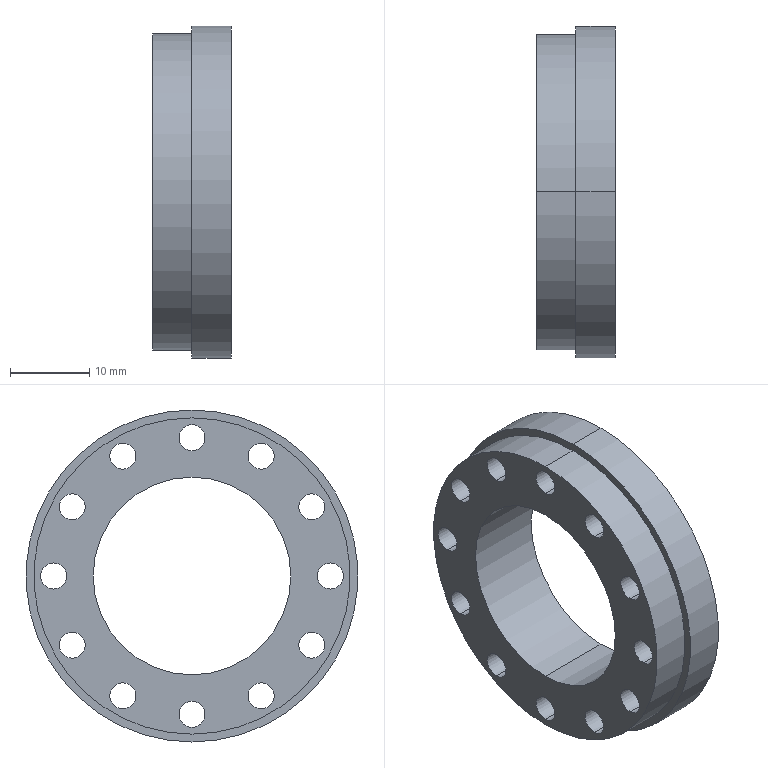Part | SolidWorks | features HoleWzd 1, Revolution 1 | 1 solid | 33 faces | box 9.95 x 42 x 42 mm | volume 7242 mm3 | cylinder 30 | plane 3 | commonest cylinder face diameters 3.3 x24 25 x2 40 x2 42 x2
STEP:
#1=CARTESIAN_POINT('',(0.,17.5,1.65));
#2=VERTEX_POINT('',#1);
#3=CARTESIAN_POINT('',(0.,17.5,-1.65));
#4=VERTEX_POINT('',#3);
#5=CARTESIAN_POINT('',(0.,17.5,0.));
#6=DIRECTION('',(1.,0.,0.));
#7=DIRECTION('',(0.,0.,-1.));
#8=AXIS2_PLACEMENT_3D('',#5,#6,#7);
#9=CIRCLE('',#8,1.65);
#10=EDGE_CURVE('',#2,#4,#9,.T.);
#11=ORIENTED_EDGE('',*,*,#10,.F.);
#12=CARTESIAN_POINT('',(9.95,17.5,1.65));
#13=VERTEX_POINT('',#12);
#14=CARTESIAN_POINT('',(9.95,17.5,1.65));
#15=DIRECTION('',(1.,0.,0.));
#16=VECTOR('',#15,1000.);
#17=LINE('',#14,#16);
#18=EDGE_CURVE('',#2,#13,#17,.T.);
#19=ORIENTED_EDGE('',*,*,#18,.T.);
#20=CARTESIAN_POINT('',(9.95,17.5,-1.65));
#21=VERTEX_POINT('',#20);
#22=CARTESIAN_POINT('',(9.95,17.5,0.));
#23=DIRECTION('',(1.,0.,0.));
#24=DIRECTION('',(0.,0.,-1.));
#25=AXIS2_PLACEMENT_3D('',#22,#23,#24);
#26=CIRCLE('',#25,1.65);
#27=EDGE_CURVE('',#13,#21,#26,.T.);
#28=ORIENTED_EDGE('',*,*,#27,.T.);
#29=CARTESIAN_POINT('',(9.95,17.5,-1.65));
#30=DIRECTION('',(1.,0.,0.));
#31=VECTOR('',#30,1000.);
#32=LINE('',#29,#31);
#33=EDGE_CURVE('',#4,#21,#32,.T.);
#34=ORIENTED_EDGE('',*,*,#33,.F.);
#35=EDGE_LOOP('',(#11,#19,#28,#34));
#36=FACE_OUTER_BOUND('',#35,.T.);
#37=CARTESIAN_POINT('',(9.95,17.5,0.));
#38=DIRECTION('',(1.,0.,0.));
#39=DIRECTION('',(0.,0.,-1.));
#40=AXIS2_PLACEMENT_3D('',#37,#38,#39);
#41=CYLINDRICAL_SURFACE('',#40,1.65);
#42=ADVANCED_FACE('',(#36),#41,.F.);
#43=CARTESIAN_POINT('',(0.,15.155,-7.1));
#44=VERTEX_POINT('',#43);
#45=CARTESIAN_POINT('',(0.,15.155,-10.4));
#46=VERTEX_POINT('',#45);
#47=CARTESIAN_POINT('',(0.,15.155,-8.75));
#48=DIRECTION('',(1.,0.,0.));
#49=DIRECTION('',(0.,0.,-1.));
#50=AXIS2_PLACEMENT_3D('',#47,#48,#49);
#51=CIRCLE('',#50,1.65);
#52=EDGE_CURVE('',#44,#46,#51,.T.);
#53=ORIENTED_EDGE('',*,*,#52,.F.);
#54=CARTESIAN_POINT('',(9.95,15.155,-7.1));
#55=VERTEX_POINT('',#54);
#56=CARTESIAN_POINT('',(9.95,15.155,-7.1));
#57=DIRECTION('',(1.,0.,0.));
#58=VECTOR('',#57,1000.);
#59=LINE('',#56,#58);
#60=EDGE_CURVE('',#44,#55,#59,.T.);
#61=ORIENTED_EDGE('',*,*,#60,.T.);
#62=CARTESIAN_POINT('',(9.95,15.155,-10.4));
#63=VERTEX_POINT('',#62);
#64=CARTESIAN_POINT('',(9.95,15.155,-8.75));
#65=DIRECTION('',(1.,0.,0.));
#66=DIRECTION('',(0.,0.,-1.));
#67=AXIS2_PLACEMENT_3D('',#64,#65,#66);
#68=CIRCLE('',#67,1.65);
#69=EDGE_CURVE('',#55,#63,#68,.T.);
#70=ORIENTED_EDGE('',*,*,#69,.T.);
#71=CARTESIAN_POINT('',(9.95,15.155,-10.4));
#72=DIRECTION('',(1.,0.,0.));
#73=VECTOR('',#72,1000.);
#74=LINE('',#71,#73);
#75=EDGE_CURVE('',#46,#63,#74,.T.);
#76=ORIENTED_EDGE('',*,*,#75,.F.);
#77=EDGE_LOOP('',(#53,#61,#70,#76));
#78=FACE_OUTER_BOUND('',#77,.T.);
#79=CARTESIAN_POINT('',(9.95,15.155,-8.75));
#80=DIRECTION('',(1.,0.,0.));
#81=DIRECTION('',(0.,0.,-1.));
#82=AXIS2_PLACEMENT_3D('',#79,#80,#81);
#83=CYLINDRICAL_SURFACE('',#82,1.65);
#84=ADVANCED_FACE('',(#78),#83,.F.);
#85=CARTESIAN_POINT('',(0.,8.75,-13.505));
#86=VERTEX_POINT('',#85);
#87=CARTESIAN_POINT('',(0.,8.75,-16.805));
#88=VERTEX_POINT('',#87);
#89=CARTESIAN_POINT('',(0.,8.75,-15.155));
#90=DIRECTION('',(1.,0.,0.));
#91=DIRECTION('',(0.,0.,-1.));
#92=AXIS2_PLACEMENT_3D('',#89,#90,#91);
#93=CIRCLE('',#92,1.65);
#94=EDGE_CURVE('',#86,#88,#93,.T.);
#95=ORIENTED_EDGE('',*,*,#94,.F.);
#96=CARTESIAN_POINT('',(9.95,8.75,-13.505));
#97=VERTEX_POINT('',#96);
#98=CARTESIAN_POINT('',(9.95,8.75,-13.505));
#99=DIRECTION('',(1.,0.,0.));
#100=VECTOR('',#99,1000.);
#101=LINE('',#98,#100);
#102=EDGE_CURVE('',#86,#97,#101,.T.);
#103=ORIENTED_EDGE('',*,*,#102,.T.);
#104=CARTESIAN_POINT('',(9.95,8.75,-16.805));
#105=VERTEX_POINT('',#104);
#106=CARTESIAN_POINT('',(9.95,8.75,-15.155));
#107=DIRECTION('',(1.,0.,0.));
#108=DIRECTION('',(0.,0.,-1.));
#109=AXIS2_PLACEMENT_3D('',#106,#107,#108);
#110=CIRCLE('',#109,1.65);
#111=EDGE_CURVE('',#97,#105,#110,.T.);
#112=ORIENTED_EDGE('',*,*,#111,.T.);
#113=CARTESIAN_POINT('',(9.95,8.75,-16.805));
#114=DIRECTION('',(1.,0.,0.));
#115=VECTOR('',#114,1000.);
#116=LINE('',#113,#115);
#117=EDGE_CURVE('',#88,#105,#116,.T.);
#118=ORIENTED_EDGE('',*,*,#117,.F.);
#119=EDGE_LOOP('',(#95,#103,#112,#118));
#120=FACE_OUTER_BOUND('',#119,.T.);
#121=CARTESIAN_POINT('',(9.95,8.75,-15.155));
#122=DIRECTION('',(1.,0.,0.));
#123=DIRECTION('',(0.,0.,-1.));
#124=AXIS2_PLACEMENT_3D('',#121,#122,#123);
#125=CYLINDRICAL_SURFACE('',#124,1.65);
#126=ADVANCED_FACE('',(#120),#125,.F.);
#127=CARTESIAN_POINT('',(0.,0.,-15.85));
#128=VERTEX_POINT('',#127);
#129=CARTESIAN_POINT('',(0.,0.,-19.15));
#130=VERTEX_POINT('',#129);
#131=CARTESIAN_POINT('',(0.,0.,-17.5));
#132=DIRECTION('',(1.,0.,0.));
#133=DIRECTION('',(0.,0.,-1.));
#134=AXIS2_PLACEMENT_3D('',#131,#132,#133);
#135=CIRCLE('',#134,1.65);
#136=EDGE_CURVE('',#128,#130,#135,.T.);
#137=ORIENTED_EDGE('',*,*,#136,.F.);
#138=CARTESIAN_POINT('',(9.95,0.,-15.85));
#139=VERTEX_POINT('',#138);
#140=CARTESIAN_POINT('',(9.95,0.,-15.85));
#141=DIRECTION('',(1.,0.,0.));
#142=VECTOR('',#141,1000.);
#143=LINE('',#140,#142);
#144=EDGE_CURVE('',#128,#139,#143,.T.);
#145=ORIENTED_EDGE('',*,*,#144,.T.);
#146=CARTESIAN_POINT('',(9.95,0.,-19.15));
#147=VERTEX_POINT('',#146);
#148=CARTESIAN_POINT('',(9.95,0.,-17.5));
#149=DIRECTION('',(1.,0.,0.));
#150=DIRECTION('',(0.,0.,-1.));
#151=AXIS2_PLACEMENT_3D('',#148,#149,#150);
#152=CIRCLE('',#151,1.65);
#153=EDGE_CURVE('',#139,#147,#152,.T.);
#154=ORIENTED_EDGE('',*,*,#153,.T.);
#155=CARTESIAN_POINT('',(9.95,0.,-19.15));
#156=DIRECTION('',(1.,0.,0.));
#157=VECTOR('',#156,1000.);
#158=LINE('',#155,#157);
#159=EDGE_CURVE('',#130,#147,#158,.T.);
#160=ORIENTED_EDGE('',*,*,#159,.F.);
#161=EDGE_LOOP('',(#137,#145,#154,#160));
#162=FACE_OUTER_BOUND('',#161,.T.);
#163=CARTESIAN_POINT('',(9.95,0.,-17.5));
#164=DIRECTION('',(1.,0.,0.));
#165=DIRECTION('',(0.,0.,-1.));
#166=AXIS2_PLACEMENT_3D('',#163,#164,#165);
#167=CYLINDRICAL_SURFACE('',#166,1.65);
#168=ADVANCED_FACE('',(#162),#167,.F.);
#169=CARTESIAN_POINT('',(0.,-8.75,-13.505));
#170=VERTEX_POINT('',#169);
#171=CARTESIAN_POINT('',(0.,-8.75,-16.805));
#172=VERTEX_POINT('',#171);
#173=CARTESIAN_POINT('',(0.,-8.75,-15.155));
#174=DIRECTION('',(1.,0.,0.));
#175=DIRECTION('',(0.,0.,-1.));
#176=AXIS2_PLACEMENT_3D('',#173,#174,#175);
#177=CIRCLE('',#176,1.65);
#178=EDGE_CURVE('',#170,#172,#177,.T.);
#179=ORIENTED_EDGE('',*,*,#178,.F.);
#180=CARTESIAN_POINT('',(9.95,-8.75,-13.505));
#181=VERTEX_POINT('',#180);
#182=CARTESIAN_POINT('',(9.95,-8.75,-13.505));
#183=DIRECTION('',(1.,0.,0.));
#184=VECTOR('',#183,1000.);
#185=LINE('',#182,#184);
#186=EDGE_CURVE('',#170,#181,#185,.T.);
#187=ORIENTED_EDGE('',*,*,#186,.T.);
#188=CARTESIAN_POINT('',(9.95,-8.75,-16.805));
#189=VERTEX_POINT('',#188);
#190=CARTESIAN_POINT('',(9.95,-8.75,-15.155));
#191=DIRECTION('',(1.,0.,0.));
#192=DIRECTION('',(0.,0.,-1.));
#193=AXIS2_PLACEMENT_3D('',#190,#191,#192);
#194=CIRCLE('',#193,1.65);
#195=EDGE_CURVE('',#181,#189,#194,.T.);
#196=ORIENTED_EDGE('',*,*,#195,.T.);
#197=CARTESIAN_POINT('',(9.95,-8.75,-16.805));
#198=DIRECTION('',(1.,0.,0.));
#199=VECTOR('',#198,1000.);
#200=LINE('',#197,#199);
#201=EDGE_CURVE('',#172,#189,#200,.T.);
#202=ORIENTED_EDGE('',*,*,#201,.F.);
#203=EDGE_LOOP('',(#179,#187,#196,#202));
#204=FACE_OUTER_BOUND('',#203,.T.);
#205=CARTESIAN_POINT('',(9.95,-8.75,-15.155));
#206=DIRECTION('',(1.,0.,0.));
#207=DIRECTION('',(0.,0.,-1.));
#208=AXIS2_PLACEMENT_3D('',#205,#206,#207);
#209=CYLINDRICAL_SURFACE('',#208,1.65);
#210=ADVANCED_FACE('',(#204),#209,.F.);
#211=CARTESIAN_POINT('',(0.,-15.155,-7.1));
#212=VERTEX_POINT('',#211);
#213=CARTESIAN_POINT('',(0.,-15.155,-10.4));
#214=VERTEX_POINT('',#213);
#215=CARTESIAN_POINT('',(0.,-15.155,-8.75));
#216=DIRECTION('',(1.,0.,0.));
#217=DIRECTION('',(0.,0.,-1.));
#218=AXIS2_PLACEMENT_3D('',#215,#216,#217);
#219=CIRCLE('',#218,1.65);
#220=EDGE_CURVE('',#212,#214,#219,.T.);
#221=ORIENTED_EDGE('',*,*,#220,.F.);
#222=CARTESIAN_POINT('',(9.95,-15.155,-7.1));
#223=VERTEX_POINT('',#222);
#224=CARTESIAN_POINT('',(9.95,-15.155,-7.1));
#225=DIRECTION('',(1.,0.,0.));
#226=VECTOR('',#225,1000.);
#227=LINE('',#224,#226);
#228=EDGE_CURVE('',#212,#223,#227,.T.);
#229=ORIENTED_EDGE('',*,*,#228,.T.);
#230=CARTESIAN_POINT('',(9.95,-15.155,-10.4));
#231=VERTEX_POINT('',#230);
#232=CARTESIAN_POINT('',(9.95,-15.155,-8.75));
#233=DIRECTION('',(1.,0.,0.));
#234=DIRECTION('',(0.,0.,-1.));
#235=AXIS2_PLACEMENT_3D('',#232,#233,#234);
#236=CIRCLE('',#235,1.65);
#237=EDGE_CURVE('',#223,#231,#236,.T.);
#238=ORIENTED_EDGE('',*,*,#237,.T.);
#239=CARTESIAN_POINT('',(9.95,-15.155,-10.4));
#240=DIRECTION('',(1.,0.,0.));
#241=VECTOR('',#240,1000.);
#242=LINE('',#239,#241);
#243=EDGE_CURVE('',#214,#231,#242,.T.);
#244=ORIENTED_EDGE('',*,*,#243,.F.);
#245=EDGE_LOOP('',(#221,#229,#238,#244));
#246=FACE_OUTER_BOUND('',#245,.T.);
#247=CARTESIAN_POINT('',(9.95,-15.155,-8.75));
#248=DIRECTION('',(1.,0.,0.));
#249=DIRECTION('',(0.,0.,-1.));
#250=AXIS2_PLACEMENT_3D('',#247,#248,#249);
#251=CYLINDRICAL_SURFACE('',#250,1.65);
#252=ADVANCED_FACE('',(#246),#251,.F.);
#253=CARTESIAN_POINT('',(0.,-17.5,1.65));
#254=VERTEX_POINT('',#253);
#255=CARTESIAN_POINT('',(0.,-17.5,-1.65));
#256=VERTEX_POINT('',#255);
#257=CARTESIAN_POINT('',(0.,-17.5,0.));
#258=DIRECTION('',(1.,0.,0.));
#259=DIRECTION('',(0.,0.,-1.));
#260=AXIS2_PLACEMENT_3D('',#257,#258,#259);
#261=CIRCLE('',#260,1.65);
#262=EDGE_CURVE('',#254,#256,#261,.T.);
#263=ORIENTED_EDGE('',*,*,#262,.F.);
#264=CARTESIAN_POINT('',(9.95,-17.5,1.65));
#265=VERTEX_POINT('',#264);
#266=CARTESIAN_POINT('',(9.95,-17.5,1.65));
#267=DIRECTION('',(1.,0.,0.));
#268=VECTOR('',#267,1000.);
#269=LINE('',#266,#268);
#270=EDGE_CURVE('',#254,#265,#269,.T.);
#271=ORIENTED_EDGE('',*,*,#270,.T.);
#272=CARTESIAN_POINT('',(9.95,-17.5,-1.65));
#273=VERTEX_POINT('',#272);
#274=CARTESIAN_POINT('',(9.95,-17.5,0.));
#275=DIRECTION('',(1.,0.,0.));
#276=DIRECTION('',(0.,0.,-1.));
#277=AXIS2_PLACEMENT_3D('',#274,#275,#276);
#278=CIRCLE('',#277,1.65);
#279=EDGE_CURVE('',#265,#273,#278,.T.);
#280=ORIENTED_EDGE('',*,*,#279,.T.);
#281=CARTESIAN_POINT('',(9.95,-17.5,-1.65));
#282=DIRECTION('',(1.,0.,0.));
#283=VECTOR('',#282,1000.);
#284=LINE('',#281,#283);
#285=EDGE_CURVE('',#256,#273,#284,.T.);
#286=ORIENTED_EDGE('',*,*,#285,.F.);
#287=EDGE_LOOP('',(#263,#271,#280,#286));
#288=FACE_OUTER_BOUND('',#287,.T.);
#289=CARTESIAN_POINT('',(9.95,-17.5,0.));
#290=DIRECTION('',(1.,0.,0.));
#291=DIRECTION('',(0.,0.,-1.));
#292=AXIS2_PLACEMENT_3D('',#289,#290,#291);
#293=CYLINDRICAL_SURFACE('',#292,1.65);
#294=ADVANCED_FACE('',(#288),#293,.F.);
#295=CARTESIAN_POINT('',(0.,-15.155,10.4));
#296=VERTEX_POINT('',#295);
#297=CARTESIAN_POINT('',(0.,-15.155,7.1));
#298=VERTEX_POINT('',#297);
#299=CARTESIAN_POINT('',(0.,-15.155,8.75));
#300=DIRECTION('',(1.,0.,0.));
#301=DIRECTION('',(0.,0.,-1.));
#302=AXIS2_PLACEMENT_3D('',#299,#300,#301);
#303=CIRCLE('',#302,1.65);
#304=EDGE_CURVE('',#296,#298,#303,.T.);
#305=ORIENTED_EDGE('',*,*,#304,.F.);
#306=CARTESIAN_POINT('',(9.95,-15.155,10.4));
#307=VERTEX_POINT('',#306);
#308=CARTESIAN_POINT('',(9.95,-15.155,10.4));
#309=DIRECTION('',(1.,0.,0.));
#310=VECTOR('',#309,1000.);
#311=LINE('',#308,#310);
#312=EDGE_CURVE('',#296,#307,#311,.T.);
#313=ORIENTED_EDGE('',*,*,#312,.T.);
#314=CARTESIAN_POINT('',(9.95,-15.155,7.1));
#315=VERTEX_POINT('',#314);
#316=CARTESIAN_POINT('',(9.95,-15.155,8.75));
#317=DIRECTION('',(1.,0.,0.));
#318=DIRECTION('',(0.,0.,-1.));
#319=AXIS2_PLACEMENT_3D('',#316,#317,#318);
#320=CIRCLE('',#319,1.65);
#321=EDGE_CURVE('',#307,#315,#320,.T.);
#322=ORIENTED_EDGE('',*,*,#321,.T.);
#323=CARTESIAN_POINT('',(9.95,-15.155,7.1));
#324=DIRECTION('',(1.,0.,0.));
#325=VECTOR('',#324,1000.);
#326=LINE('',#323,#325);
#327=EDGE_CURVE('',#298,#315,#326,.T.);
#328=ORIENTED_EDGE('',*,*,#327,.F.);
#329=EDGE_LOOP('',(#305,#313,#322,#328));
#330=FACE_OUTER_BOUND('',#329,.T.);
#331=CARTESIAN_POINT('',(9.95,-15.155,8.75));
#332=DIRECTION('',(1.,0.,0.));
#333=DIRECTION('',(0.,0.,-1.));
#334=AXIS2_PLACEMENT_3D('',#331,#332,#333);
#335=CYLINDRICAL_SURFACE('',#334,1.65);
#336=ADVANCED_FACE('',(#330),#335,.F.);
#337=CARTESIAN_POINT('',(0.,-8.75,16.805));
#338=VERTEX_POINT('',#337);
#339=CARTESIAN_POINT('',(0.,-8.75,13.505));
#340=VERTEX_POINT('',#339);
#341=CARTESIAN_POINT('',(0.,-8.75,15.155));
#342=DIRECTION('',(1.,0.,0.));
#343=DIRECTION('',(0.,0.,-1.));
#344=AXIS2_PLACEMENT_3D('',#341,#342,#343);
#345=CIRCLE('',#344,1.65);
#346=EDGE_CURVE('',#338,#340,#345,.T.);
#347=ORIENTED_EDGE('',*,*,#346,.F.);
#348=CARTESIAN_POINT('',(9.95,-8.75,16.805));
#349=VERTEX_POINT('',#348);
#350=CARTESIAN_POINT('',(9.95,-8.75,16.805));
#351=DIRECTION('',(1.,0.,0.));
#352=VECTOR('',#351,1000.);
#353=LINE('',#350,#352);
#354=EDGE_CURVE('',#338,#349,#353,.T.);
#355=ORIENTED_EDGE('',*,*,#354,.T.);
#356=CARTESIAN_POINT('',(9.95,-8.75,13.505));
#357=VERTEX_POINT('',#356);
#358=CARTESIAN_POINT('',(9.95,-8.75,15.155));
#359=DIRECTION('',(1.,0.,0.));
#360=DIRECTION('',(0.,0.,-1.));
#361=AXIS2_PLACEMENT_3D('',#358,#359,#360);
#362=CIRCLE('',#361,1.65);
#363=EDGE_CURVE('',#349,#357,#362,.T.);
#364=ORIENTED_EDGE('',*,*,#363,.T.);
#365=CARTESIAN_POINT('',(9.95,-8.75,13.505));
#366=DIRECTION('',(1.,0.,0.));
#367=VECTOR('',#366,1000.);
#368=LINE('',#365,#367);
#369=EDGE_CURVE('',#340,#357,#368,.T.);
#370=ORIENTED_EDGE('',*,*,#369,.F.);
#371=EDGE_LOOP('',(#347,#355,#364,#370));
#372=FACE_OUTER_BOUND('',#371,.T.);
#373=CARTESIAN_POINT('',(9.95,-8.75,15.155));
#374=DIRECTION('',(1.,0.,0.));
#375=DIRECTION('',(0.,0.,-1.));
#376=AXIS2_PLACEMENT_3D('',#373,#374,#375);
#377=CYLINDRICAL_SURFACE('',#376,1.65);
#378=ADVANCED_FACE('',(#372),#377,.F.);
#379=CARTESIAN_POINT('',(0.,0.,19.15));
#380=VERTEX_POINT('',#379);
#381=CARTESIAN_POINT('',(0.,0.,15.85));
#382=VERTEX_POINT('',#381);
#383=CARTESIAN_POINT('',(0.,0.,17.5));
#384=DIRECTION('',(1.,0.,0.));
#385=DIRECTION('',(0.,0.,-1.));
#386=AXIS2_PLACEMENT_3D('',#383,#384,#385);
#387=CIRCLE('',#386,1.65);
#388=EDGE_CURVE('',#380,#382,#387,.T.);
#389=ORIENTED_EDGE('',*,*,#388,.F.);
#390=CARTESIAN_POINT('',(9.95,0.,19.15));
#391=VERTEX_POINT('',#390);
#392=CARTESIAN_POINT('',(9.95,0.,19.15));
#393=DIRECTION('',(1.,0.,0.));
#394=VECTOR('',#393,1000.);
#395=LINE('',#392,#394);
#396=EDGE_CURVE('',#380,#391,#395,.T.);
#397=ORIENTED_EDGE('',*,*,#396,.T.);
#398=CARTESIAN_POINT('',(9.95,0.,15.85));
#399=VERTEX_POINT('',#398);
#400=CARTESIAN_POINT('',(9.95,0.,17.5));
#401=DIRECTION('',(1.,0.,0.));
#402=DIRECTION('',(0.,0.,-1.));
#403=AXIS2_PLACEMENT_3D('',#400,#401,#402);
#404=CIRCLE('',#403,1.65);
#405=EDGE_CURVE('',#391,#399,#404,.T.);
#406=ORIENTED_EDGE('',*,*,#405,.T.);
#407=CARTESIAN_POINT('',(9.95,0.,15.85));
#408=DIRECTION('',(1.,0.,0.));
#409=VECTOR('',#408,1000.);
#410=LINE('',#407,#409);
#411=EDGE_CURVE('',#382,#399,#410,.T.);
#412=ORIENTED_EDGE('',*,*,#411,.F.);
#413=EDGE_LOOP('',(#389,#397,#406,#412));
#414=FACE_OUTER_BOUND('',#413,.T.);
#415=CARTESIAN_POINT('',(9.95,0.,17.5));
#416=DIRECTION('',(1.,0.,0.));
#417=DIRECTION('',(0.,0.,-1.));
#418=AXIS2_PLACEMENT_3D('',#415,#416,#417);
#419=CYLINDRICAL_SURFACE('',#418,1.65);
#420=ADVANCED_FACE('',(#414),#419,.F.);
#421=CARTESIAN_POINT('',(0.,8.75,16.805));
#422=VERTEX_POINT('',#421);
#423=CARTESIAN_POINT('',(0.,8.75,13.505));
#424=VERTEX_POINT('',#423);
#425=CARTESIAN_POINT('',(0.,8.75,15.155));
#426=DIRECTION('',(1.,0.,0.));
#427=DIRECTION('',(0.,0.,-1.));
#428=AXIS2_PLACEMENT_3D('',#425,#426,#427);
#429=CIRCLE('',#428,1.65);
#430=EDGE_CURVE('',#422,#424,#429,.T.);
#431=ORIENTED_EDGE('',*,*,#430,.F.);
#432=CARTESIAN_POINT('',(9.95,8.75,16.805));
#433=VERTEX_POINT('',#432);
#434=CARTESIAN_POINT('',(9.95,8.75,16.805));
#435=DIRECTION('',(1.,0.,0.));
#436=VECTOR('',#435,1000.);
#437=LINE('',#434,#436);
#438=EDGE_CURVE('',#422,#433,#437,.T.);
#439=ORIENTED_EDGE('',*,*,#438,.T.);
#440=CARTESIAN_POINT('',(9.95,8.75,13.505));
#441=VERTEX_POINT('',#440);
#442=CARTESIAN_POINT('',(9.95,8.75,15.155));
#443=DIRECTION('',(1.,0.,0.));
#444=DIRECTION('',(0.,0.,-1.));
#445=AXIS2_PLACEMENT_3D('',#442,#443,#444);
#446=CIRCLE('',#445,1.65);
#447=EDGE_CURVE('',#433,#441,#446,.T.);
#448=ORIENTED_EDGE('',*,*,#447,.T.);
#449=CARTESIAN_POINT('',(9.95,8.75,13.505));
#450=DIRECTION('',(1.,0.,0.));
#451=VECTOR('',#450,1000.);
#452=LINE('',#449,#451);
#453=EDGE_CURVE('',#424,#441,#452,.T.);
#454=ORIENTED_EDGE('',*,*,#453,.F.);
#455=EDGE_LOOP('',(#431,#439,#448,#454));
#456=FACE_OUTER_BOUND('',#455,.T.);
#457=CARTESIAN_POINT('',(9.95,8.75,15.155));
#458=DIRECTION('',(1.,0.,0.));
#459=DIRECTION('',(0.,0.,-1.));
#460=AXIS2_PLACEMENT_3D('',#457,#458,#459);
#461=CYLINDRICAL_SURFACE('',#460,1.65);
#462=ADVANCED_FACE('',(#456),#461,.F.);
#463=CARTESIAN_POINT('',(0.,15.155,10.4));
#464=VERTEX_POINT('',#463);
#465=CARTESIAN_POINT('',(0.,15.155,7.1));
#466=VERTEX_POINT('',#465);
#467=CARTESIAN_POINT('',(0.,15.155,8.75));
#468=DIRECTION('',(1.,0.,0.));
#469=DIRECTION('',(0.,0.,-1.));
#470=AXIS2_PLACEMENT_3D('',#467,#468,#469);
#471=CIRCLE('',#470,1.65);
#472=EDGE_CURVE('',#464,#466,#471,.T.);
#473=ORIENTED_EDGE('',*,*,#472,.F.);
#474=CARTESIAN_POINT('',(9.95,15.155,10.4));
#475=VERTEX_POINT('',#474);
#476=CARTESIAN_POINT('',(9.95,15.155,10.4));
#477=DIRECTION('',(1.,0.,0.));
#478=VECTOR('',#477,1000.);
#479=LINE('',#476,#478);
#480=EDGE_CURVE('',#464,#475,#479,.T.);
#481=ORIENTED_EDGE('',*,*,#480,.T.);
#482=CARTESIAN_POINT('',(9.95,15.155,7.1));
#483=VERTEX_POINT('',#482);
#484=CARTESIAN_POINT('',(9.95,15.155,8.75));
#485=DIRECTION('',(1.,0.,0.));
#486=DIRECTION('',(0.,0.,-1.));
#487=AXIS2_PLACEMENT_3D('',#484,#485,#486);
#488=CIRCLE('',#487,1.65);
#489=EDGE_CURVE('',#475,#483,#488,.T.);
#490=ORIENTED_EDGE('',*,*,#489,.T.);
#491=CARTESIAN_POINT('',(9.95,15.155,7.1));
#492=DIRECTION('',(1.,0.,0.));
#493=VECTOR('',#492,1000.);
#494=LINE('',#491,#493);
#495=EDGE_CURVE('',#466,#483,#494,.T.);
#496=ORIENTED_EDGE('',*,*,#495,.F.);
#497=EDGE_LOOP('',(#473,#481,#490,#496));
#498=FACE_OUTER_BOUND('',#497,.T.);
#499=CARTESIAN_POINT('',(9.95,15.155,8.75));
#500=DIRECTION('',(1.,0.,0.));
#501=DIRECTION('',(0.,0.,-1.));
#502=AXIS2_PLACEMENT_3D('',#499,#500,#501);
#503=CYLINDRICAL_SURFACE('',#502,1.65);
#504=ADVANCED_FACE('',(#498),#503,.F.);
#505=CARTESIAN_POINT('',(9.95,0.,21.));
#506=VERTEX_POINT('',#505);
#507=CARTESIAN_POINT('',(9.95,0.,-21.));
#508=VERTEX_POINT('',#507);
#509=CARTESIAN_POINT('',(9.95,0.,0.));
#510=DIRECTION('',(-1.,0.,0.));
#511=DIRECTION('',(0.,0.,1.));
#512=AXIS2_PLACEMENT_3D('',#509,#510,#511);
#513=CIRCLE('',#512,21.);
#514=EDGE_CURVE('',#506,#508,#513,.T.);
#515=ORIENTED_EDGE('',*,*,#514,.T.);
#516=CARTESIAN_POINT('',(4.95,0.,-21.));
#517=VERTEX_POINT('',#516);
#518=CARTESIAN_POINT('',(-63.944,0.,-21.));
#519=DIRECTION('',(-1.,0.,0.));
#520=VECTOR('',#519,1000.);
#521=LINE('',#518,#520);
#522=EDGE_CURVE('',#508,#517,#521,.T.);
#523=ORIENTED_EDGE('',*,*,#522,.T.);
#524=CARTESIAN_POINT('',(4.95,0.,21.));
#525=VERTEX_POINT('',#524);
#526=CARTESIAN_POINT('',(4.95,0.,0.));
#527=DIRECTION('',(-1.,0.,0.));
#528=DIRECTION('',(0.,0.,1.));
#529=AXIS2_PLACEMENT_3D('',#526,#527,#528);
#530=CIRCLE('',#529,21.);
#531=EDGE_CURVE('',#525,#517,#530,.T.);
#532=ORIENTED_EDGE('',*,*,#531,.F.);
#533=CARTESIAN_POINT('',(-63.944,0.,21.));
#534=DIRECTION('',(-1.,0.,0.));
#535=VECTOR('',#534,1000.);
#536=LINE('',#533,#535);
#537=EDGE_CURVE('',#506,#525,#536,.T.);
#538=ORIENTED_EDGE('',*,*,#537,.F.);
#539=EDGE_LOOP('',(#515,#523,#532,#538));
#540=FACE_OUTER_BOUND('',#539,.T.);
#541=CARTESIAN_POINT('',(-63.944,0.,0.));
#542=DIRECTION('',(-1.,0.,0.));
#543=DIRECTION('',(0.,0.,1.));
#544=AXIS2_PLACEMENT_3D('',#541,#542,#543);
#545=CYLINDRICAL_SURFACE('',#544,21.);
#546=ADVANCED_FACE('',(#540),#545,.T.);
#547=CARTESIAN_POINT('',(4.95,0.,20.));
#548=VERTEX_POINT('',#547);
#549=CARTESIAN_POINT('',(4.95,0.,-20.));
#550=VERTEX_POINT('',#549);
#551=CARTESIAN_POINT('',(4.95,0.,0.));
#552=DIRECTION('',(-1.,0.,0.));
#553=DIRECTION('',(0.,0.,1.));
#554=AXIS2_PLACEMENT_3D('',#551,#552,#553);
#555=CIRCLE('',#554,20.);
#556=EDGE_CURVE('',#548,#550,#555,.T.);
#557=ORIENTED_EDGE('',*,*,#556,.T.);
#558=CARTESIAN_POINT('',(0.,0.,-20.));
#559=VERTEX_POINT('',#558);
#560=CARTESIAN_POINT('',(-63.944,0.,-20.));
#561=DIRECTION('',(-1.,0.,0.));
#562=VECTOR('',#561,1000.);
#563=LINE('',#560,#562);
#564=EDGE_CURVE('',#550,#559,#563,.T.);
#565=ORIENTED_EDGE('',*,*,#564,.T.);
#566=CARTESIAN_POINT('',(0.,0.,20.));
#567=VERTEX_POINT('',#566);
#568=CARTESIAN_POINT('',(0.,0.,0.));
#569=DIRECTION('',(-1.,0.,0.));
#570=DIRECTION('',(0.,0.,1.));
#571=AXIS2_PLACEMENT_3D('',#568,#569,#570);
#572=CIRCLE('',#571,20.);
#573=EDGE_CURVE('',#567,#559,#572,.T.);
#574=ORIENTED_EDGE('',*,*,#573,.F.);
#575=CARTESIAN_POINT('',(-63.944,0.,20.));
#576=DIRECTION('',(-1.,0.,0.));
#577=VECTOR('',#576,1000.);
#578=LINE('',#575,#577);
#579=EDGE_CURVE('',#548,#567,#578,.T.);
#580=ORIENTED_EDGE('',*,*,#579,.F.);
#581=EDGE_LOOP('',(#557,#565,#574,#580));
#582=FACE_OUTER_BOUND('',#581,.T.);
#583=CARTESIAN_POINT('',(-63.944,0.,0.));
#584=DIRECTION('',(-1.,0.,0.));
#585=DIRECTION('',(0.,0.,1.));
#586=AXIS2_PLACEMENT_3D('',#583,#584,#585);
#587=CYLINDRICAL_SURFACE('',#586,20.);
#588=ADVANCED_FACE('',(#582),#587,.T.);
#589=CARTESIAN_POINT('',(9.95,0.,-12.5));
#590=VERTEX_POINT('',#589);
#591=CARTESIAN_POINT('',(9.95,0.,12.5));
#592=VERTEX_POINT('',#591);
#593=CARTESIAN_POINT('',(9.95,0.,0.));
#594=DIRECTION('',(-1.,0.,0.));
#595=DIRECTION('',(0.,0.,1.));
#596=AXIS2_PLACEMENT_3D('',#593,#594,#595);
#597=CIRCLE('',#596,12.5);
#598=EDGE_CURVE('',#590,#592,#597,.T.);
#599=ORIENTED_EDGE('',*,*,#598,.F.);
#600=CARTESIAN_POINT('',(0.,0.,-12.5));
#601=VERTEX_POINT('',#600);
#602=CARTESIAN_POINT('',(-63.944,0.,-12.5));
#603=DIRECTION('',(-1.,0.,0.));
#604=VECTOR('',#603,1000.);
#605=LINE('',#602,#604);
#606=EDGE_CURVE('',#590,#601,#605,.T.);
#607=ORIENTED_EDGE('',*,*,#606,.T.);
#608=CARTESIAN_POINT('',(0.,0.,12.5));
#609=VERTEX_POINT('',#608);
#610=CARTESIAN_POINT('',(0.,0.,0.));
#611=DIRECTION('',(-1.,0.,0.));
#612=DIRECTION('',(0.,0.,1.));
#613=AXIS2_PLACEMENT_3D('',#610,#611,#612);
#614=CIRCLE('',#613,12.5);
#615=EDGE_CURVE('',#601,#609,#614,.T.);
#616=ORIENTED_EDGE('',*,*,#615,.T.);
#617=CARTESIAN_POINT('',(-63.944,0.,12.5));
#618=DIRECTION('',(-1.,0.,0.));
#619=VECTOR('',#618,1000.);
#620=LINE('',#617,#619);
#621=EDGE_CURVE('',#592,#609,#620,.T.);
#622=ORIENTED_EDGE('',*,*,#621,.F.);
#623=EDGE_LOOP('',(#599,#607,#616,#622));
#624=FACE_OUTER_BOUND('',#623,.T.);
#625=CARTESIAN_POINT('',(-63.944,0.,0.));
#626=DIRECTION('',(-1.,0.,0.));
#627=DIRECTION('',(0.,0.,1.));
#628=AXIS2_PLACEMENT_3D('',#625,#626,#627);
#629=CYLINDRICAL_SURFACE('',#628,12.5);
#630=ADVANCED_FACE('',(#624),#629,.F.);
#631=CARTESIAN_POINT('',(9.95,15.155,-8.75));
#632=DIRECTION('',(1.,0.,0.));
#633=DIRECTION('',(0.,0.,-1.));
#634=AXIS2_PLACEMENT_3D('',#631,#632,#633);
#635=CIRCLE('',#634,1.65);
#636=EDGE_CURVE('',#63,#55,#635,.T.);
#637=ORIENTED_EDGE('',*,*,#636,.F.);
#638=ORIENTED_EDGE('',*,*,#69,.F.);
#639=EDGE_LOOP('',(#637,#638));
#640=FACE_BOUND('',#639,.T.);
#641=CARTESIAN_POINT('',(9.95,8.75,-15.155));
#642=DIRECTION('',(1.,0.,0.));
#643=DIRECTION('',(0.,0.,-1.));
#644=AXIS2_PLACEMENT_3D('',#641,#642,#643);
#645=CIRCLE('',#644,1.65);
#646=EDGE_CURVE('',#105,#97,#645,.T.);
#647=ORIENTED_EDGE('',*,*,#646,.F.);
#648=ORIENTED_EDGE('',*,*,#111,.F.);
#649=EDGE_LOOP('',(#647,#648));
#650=FACE_BOUND('',#649,.T.);
#651=CARTESIAN_POINT('',(9.95,0.,-17.5));
#652=DIRECTION('',(1.,0.,0.));
#653=DIRECTION('',(0.,0.,-1.));
#654=AXIS2_PLACEMENT_3D('',#651,#652,#653);
#655=CIRCLE('',#654,1.65);
#656=EDGE_CURVE('',#147,#139,#655,.T.);
#657=ORIENTED_EDGE('',*,*,#656,.F.);
#658=ORIENTED_EDGE('',*,*,#153,.F.);
#659=EDGE_LOOP('',(#657,#658));
#660=FACE_BOUND('',#659,.T.);
#661=CARTESIAN_POINT('',(9.95,-8.75,-15.155));
#662=DIRECTION('',(1.,0.,0.));
#663=DIRECTION('',(0.,0.,-1.));
#664=AXIS2_PLACEMENT_3D('',#661,#662,#663);
#665=CIRCLE('',#664,1.65);
#666=EDGE_CURVE('',#189,#181,#665,.T.);
#667=ORIENTED_EDGE('',*,*,#666,.F.);
#668=ORIENTED_EDGE('',*,*,#195,.F.);
#669=EDGE_LOOP('',(#667,#668));
#670=FACE_BOUND('',#669,.T.);
#671=CARTESIAN_POINT('',(9.95,-15.155,-8.75));
#672=DIRECTION('',(1.,0.,0.));
#673=DIRECTION('',(0.,0.,-1.));
#674=AXIS2_PLACEMENT_3D('',#671,#672,#673);
#675=CIRCLE('',#674,1.65);
#676=EDGE_CURVE('',#231,#223,#675,.T.);
#677=ORIENTED_EDGE('',*,*,#676,.F.);
#678=ORIENTED_EDGE('',*,*,#237,.F.);
#679=EDGE_LOOP('',(#677,#678));
#680=FACE_BOUND('',#679,.T.);
#681=CARTESIAN_POINT('',(9.95,-17.5,0.));
#682=DIRECTION('',(1.,0.,0.));
#683=DIRECTION('',(0.,0.,-1.));
#684=AXIS2_PLACEMENT_3D('',#681,#682,#683);
#685=CIRCLE('',#684,1.65);
#686=EDGE_CURVE('',#273,#265,#685,.T.);
#687=ORIENTED_EDGE('',*,*,#686,.F.);
#688=ORIENTED_EDGE('',*,*,#279,.F.);
#689=EDGE_LOOP('',(#687,#688));
#690=FACE_BOUND('',#689,.T.);
#691=CARTESIAN_POINT('',(9.95,-15.155,8.75));
#692=DIRECTION('',(1.,0.,0.));
#693=DIRECTION('',(0.,0.,-1.));
#694=AXIS2_PLACEMENT_3D('',#691,#692,#693);
#695=CIRCLE('',#694,1.65);
#696=EDGE_CURVE('',#315,#307,#695,.T.);
#697=ORIENTED_EDGE('',*,*,#696,.F.);
#698=ORIENTED_EDGE('',*,*,#321,.F.);
#699=EDGE_LOOP('',(#697,#698));
#700=FACE_BOUND('',#699,.T.);
#701=CARTESIAN_POINT('',(9.95,-8.75,15.155));
#702=DIRECTION('',(1.,0.,0.));
#703=DIRECTION('',(0.,0.,-1.));
#704=AXIS2_PLACEMENT_3D('',#701,#702,#703);
#705=CIRCLE('',#704,1.65);
#706=EDGE_CURVE('',#357,#349,#705,.T.);
#707=ORIENTED_EDGE('',*,*,#706,.F.);
#708=ORIENTED_EDGE('',*,*,#363,.F.);
#709=EDGE_LOOP('',(#707,#708));
#710=FACE_BOUND('',#709,.T.);
#711=CARTESIAN_POINT('',(9.95,0.,17.5));
#712=DIRECTION('',(1.,0.,0.));
#713=DIRECTION('',(0.,0.,-1.));
#714=AXIS2_PLACEMENT_3D('',#711,#712,#713);
#715=CIRCLE('',#714,1.65);
#716=EDGE_CURVE('',#399,#391,#715,.T.);
#717=ORIENTED_EDGE('',*,*,#716,.F.);
#718=ORIENTED_EDGE('',*,*,#405,.F.);
#719=EDGE_LOOP('',(#717,#718));
#720=FACE_BOUND('',#719,.T.);
#721=CARTESIAN_POINT('',(9.95,8.75,15.155));
#722=DIRECTION('',(1.,0.,0.));
#723=DIRECTION('',(0.,0.,-1.));
#724=AXIS2_PLACEMENT_3D('',#721,#722,#723);
#725=CIRCLE('',#724,1.65);
#726=EDGE_CURVE('',#441,#433,#725,.T.);
#727=ORIENTED_EDGE('',*,*,#726,.F.);
#728=ORIENTED_EDGE('',*,*,#447,.F.);
#729=EDGE_LOOP('',(#727,#728));
#730=FACE_BOUND('',#729,.T.);
#731=CARTESIAN_POINT('',(9.95,15.155,8.75));
#732=DIRECTION('',(1.,0.,0.));
#733=DIRECTION('',(0.,0.,-1.));
#734=AXIS2_PLACEMENT_3D('',#731,#732,#733);
#735=CIRCLE('',#734,1.65);
#736=EDGE_CURVE('',#483,#475,#735,.T.);
#737=ORIENTED_EDGE('',*,*,#736,.F.);
#738=ORIENTED_EDGE('',*,*,#489,.F.);
#739=EDGE_LOOP('',(#737,#738));
#740=FACE_BOUND('',#739,.T.);
#741=ORIENTED_EDGE('',*,*,#514,.F.);
#742=CARTESIAN_POINT('',(9.95,0.,0.));
#743=DIRECTION('',(-1.,0.,0.));
#744=DIRECTION('',(0.,0.,1.));
#745=AXIS2_PLACEMENT_3D('',#742,#743,#744);
#746=CIRCLE('',#745,21.);
#747=EDGE_CURVE('',#508,#506,#746,.T.);
#748=ORIENTED_EDGE('',*,*,#747,.F.);
#749=EDGE_LOOP('',(#741,#748));
#750=FACE_OUTER_BOUND('',#749,.T.);
#751=CARTESIAN_POINT('',(9.95,0.,0.));
#752=DIRECTION('',(-1.,0.,0.));
#753=DIRECTION('',(0.,0.,1.));
#754=AXIS2_PLACEMENT_3D('',#751,#752,#753);
#755=CIRCLE('',#754,12.5);
#756=EDGE_CURVE('',#592,#590,#755,.T.);
#757=ORIENTED_EDGE('',*,*,#756,.T.);
#758=ORIENTED_EDGE('',*,*,#598,.T.);
#759=EDGE_LOOP('',(#757,#758));
#760=FACE_BOUND('',#759,.T.);
#761=CARTESIAN_POINT('',(9.95,17.5,0.));
#762=DIRECTION('',(1.,0.,0.));
#763=DIRECTION('',(0.,0.,-1.));
#764=AXIS2_PLACEMENT_3D('',#761,#762,#763);
#765=CIRCLE('',#764,1.65);
#766=EDGE_CURVE('',#21,#13,#765,.T.);
#767=ORIENTED_EDGE('',*,*,#766,.F.);
#768=ORIENTED_EDGE('',*,*,#27,.F.);
#769=EDGE_LOOP('',(#767,#768));
#770=FACE_BOUND('',#769,.T.);
#771=CARTESIAN_POINT('',(9.95,0.,-21.));
#772=DIRECTION('',(-1.,0.,0.));
#773=DIRECTION('',(0.,0.,1.));
#774=AXIS2_PLACEMENT_3D('',#771,#772,#773);
#775=PLANE('',#774);
#776=ADVANCED_FACE('',(#640,#650,#660,#670,#680,#690,#700,#710,#720,#730,#740,#750,#760,#770),#775,.F.);
#777=ORIENTED_EDGE('',*,*,#606,.F.);
#778=ORIENTED_EDGE('',*,*,#756,.F.);
#779=ORIENTED_EDGE('',*,*,#621,.T.);
#780=CARTESIAN_POINT('',(0.,0.,0.));
#781=DIRECTION('',(-1.,0.,0.));
#782=DIRECTION('',(0.,0.,1.));
#783=AXIS2_PLACEMENT_3D('',#780,#781,#782);
#784=CIRCLE('',#783,12.5);
#785=EDGE_CURVE('',#609,#601,#784,.T.);
#786=ORIENTED_EDGE('',*,*,#785,.T.);
#787=EDGE_LOOP('',(#777,#778,#779,#786));
#788=FACE_OUTER_BOUND('',#787,.T.);
#789=CARTESIAN_POINT('',(-63.944,0.,0.));
#790=DIRECTION('',(-1.,0.,0.));
#791=DIRECTION('',(0.,0.,1.));
#792=AXIS2_PLACEMENT_3D('',#789,#790,#791);
#793=CYLINDRICAL_SURFACE('',#792,12.5);
#794=ADVANCED_FACE('',(#788),#793,.F.);
#795=CARTESIAN_POINT('',(0.,17.5,0.));
#796=DIRECTION('',(1.,0.,0.));
#797=DIRECTION('',(0.,0.,-1.));
#798=AXIS2_PLACEMENT_3D('',#795,#796,#797);
#799=CIRCLE('',#798,1.65);
#800=EDGE_CURVE('',#4,#2,#799,.T.);
#801=ORIENTED_EDGE('',*,*,#800,.T.);
#802=ORIENTED_EDGE('',*,*,#10,.T.);
#803=EDGE_LOOP('',(#801,#802));
#804=FACE_BOUND('',#803,.T.);
#805=CARTESIAN_POINT('',(0.,15.155,-8.75));
#806=DIRECTION('',(1.,0.,0.));
#807=DIRECTION('',(0.,0.,-1.));
#808=AXIS2_PLACEMENT_3D('',#805,#806,#807);
#809=CIRCLE('',#808,1.65);
#810=EDGE_CURVE('',#46,#44,#809,.T.);
#811=ORIENTED_EDGE('',*,*,#810,.T.);
#812=ORIENTED_EDGE('',*,*,#52,.T.);
#813=EDGE_LOOP('',(#811,#812));
#814=FACE_BOUND('',#813,.T.);
#815=CARTESIAN_POINT('',(0.,8.75,-15.155));
#816=DIRECTION('',(1.,0.,0.));
#817=DIRECTION('',(0.,0.,-1.));
#818=AXIS2_PLACEMENT_3D('',#815,#816,#817);
#819=CIRCLE('',#818,1.65);
#820=EDGE_CURVE('',#88,#86,#819,.T.);
#821=ORIENTED_EDGE('',*,*,#820,.T.);
#822=ORIENTED_EDGE('',*,*,#94,.T.);
#823=EDGE_LOOP('',(#821,#822));
#824=FACE_BOUND('',#823,.T.);
#825=CARTESIAN_POINT('',(0.,0.,-17.5));
#826=DIRECTION('',(1.,0.,0.));
#827=DIRECTION('',(0.,0.,-1.));
#828=AXIS2_PLACEMENT_3D('',#825,#826,#827);
#829=CIRCLE('',#828,1.65);
#830=EDGE_CURVE('',#130,#128,#829,.T.);
#831=ORIENTED_EDGE('',*,*,#830,.T.);
#832=ORIENTED_EDGE('',*,*,#136,.T.);
#833=EDGE_LOOP('',(#831,#832));
#834=FACE_BOUND('',#833,.T.);
#835=CARTESIAN_POINT('',(0.,-8.75,-15.155));
#836=DIRECTION('',(1.,0.,0.));
#837=DIRECTION('',(0.,0.,-1.));
#838=AXIS2_PLACEMENT_3D('',#835,#836,#837);
#839=CIRCLE('',#838,1.65);
#840=EDGE_CURVE('',#172,#170,#839,.T.);
#841=ORIENTED_EDGE('',*,*,#840,.T.);
#842=ORIENTED_EDGE('',*,*,#178,.T.);
#843=EDGE_LOOP('',(#841,#842));
#844=FACE_BOUND('',#843,.T.);
#845=CARTESIAN_POINT('',(0.,-15.155,-8.75));
#846=DIRECTION('',(1.,0.,0.));
#847=DIRECTION('',(0.,0.,-1.));
#848=AXIS2_PLACEMENT_3D('',#845,#846,#847);
#849=CIRCLE('',#848,1.65);
#850=EDGE_CURVE('',#214,#212,#849,.T.);
#851=ORIENTED_EDGE('',*,*,#850,.T.);
#852=ORIENTED_EDGE('',*,*,#220,.T.);
#853=EDGE_LOOP('',(#851,#852));
#854=FACE_BOUND('',#853,.T.);
#855=CARTESIAN_POINT('',(0.,-17.5,0.));
#856=DIRECTION('',(1.,0.,0.));
#857=DIRECTION('',(0.,0.,-1.));
#858=AXIS2_PLACEMENT_3D('',#855,#856,#857);
#859=CIRCLE('',#858,1.65);
#860=EDGE_CURVE('',#256,#254,#859,.T.);
#861=ORIENTED_EDGE('',*,*,#860,.T.);
#862=ORIENTED_EDGE('',*,*,#262,.T.);
#863=EDGE_LOOP('',(#861,#862));
#864=FACE_BOUND('',#863,.T.);
#865=CARTESIAN_POINT('',(0.,-15.155,8.75));
#866=DIRECTION('',(1.,0.,0.));
#867=DIRECTION('',(0.,0.,-1.));
#868=AXIS2_PLACEMENT_3D('',#865,#866,#867);
#869=CIRCLE('',#868,1.65);
#870=EDGE_CURVE('',#298,#296,#869,.T.);
#871=ORIENTED_EDGE('',*,*,#870,.T.);
#872=ORIENTED_EDGE('',*,*,#304,.T.);
#873=EDGE_LOOP('',(#871,#872));
#874=FACE_BOUND('',#873,.T.);
#875=CARTESIAN_POINT('',(0.,-8.75,15.155));
#876=DIRECTION('',(1.,0.,0.));
#877=DIRECTION('',(0.,0.,-1.));
#878=AXIS2_PLACEMENT_3D('',#875,#876,#877);
#879=CIRCLE('',#878,1.65);
#880=EDGE_CURVE('',#340,#338,#879,.T.);
#881=ORIENTED_EDGE('',*,*,#880,.T.);
#882=ORIENTED_EDGE('',*,*,#346,.T.);
#883=EDGE_LOOP('',(#881,#882));
#884=FACE_BOUND('',#883,.T.);
#885=CARTESIAN_POINT('',(0.,0.,17.5));
#886=DIRECTION('',(1.,0.,0.));
#887=DIRECTION('',(0.,0.,-1.));
#888=AXIS2_PLACEMENT_3D('',#885,#886,#887);
#889=CIRCLE('',#888,1.65);
#890=EDGE_CURVE('',#382,#380,#889,.T.);
#891=ORIENTED_EDGE('',*,*,#890,.T.);
#892=ORIENTED_EDGE('',*,*,#388,.T.);
#893=EDGE_LOOP('',(#891,#892));
#894=FACE_BOUND('',#893,.T.);
#895=CARTESIAN_POINT('',(0.,8.75,15.155));
#896=DIRECTION('',(1.,0.,0.));
#897=DIRECTION('',(0.,0.,-1.));
#898=AXIS2_PLACEMENT_3D('',#895,#896,#897);
#899=CIRCLE('',#898,1.65);
#900=EDGE_CURVE('',#424,#422,#899,.T.);
#901=ORIENTED_EDGE('',*,*,#900,.T.);
#902=ORIENTED_EDGE('',*,*,#430,.T.);
#903=EDGE_LOOP('',(#901,#902));
#904=FACE_BOUND('',#903,.T.);
#905=CARTESIAN_POINT('',(0.,15.155,8.75));
#906=DIRECTION('',(1.,0.,0.));
#907=DIRECTION('',(0.,0.,-1.));
#908=AXIS2_PLACEMENT_3D('',#905,#906,#907);
#909=CIRCLE('',#908,1.65);
#910=EDGE_CURVE('',#466,#464,#909,.T.);
#911=ORIENTED_EDGE('',*,*,#910,.T.);
#912=ORIENTED_EDGE('',*,*,#472,.T.);
#913=EDGE_LOOP('',(#911,#912));
#914=FACE_BOUND('',#913,.T.);
#915=ORIENTED_EDGE('',*,*,#785,.F.);
#916=ORIENTED_EDGE('',*,*,#615,.F.);
#917=EDGE_LOOP('',(#915,#916));
#918=FACE_BOUND('',#917,.T.);
#919=ORIENTED_EDGE('',*,*,#573,.T.);
#920=CARTESIAN_POINT('',(0.,0.,0.));
#921=DIRECTION('',(-1.,0.,0.));
#922=DIRECTION('',(0.,0.,1.));
#923=AXIS2_PLACEMENT_3D('',#920,#921,#922);
#924=CIRCLE('',#923,20.);
#925=EDGE_CURVE('',#559,#567,#924,.T.);
#926=ORIENTED_EDGE('',*,*,#925,.T.);
#927=EDGE_LOOP('',(#919,#926));
#928=FACE_OUTER_BOUND('',#927,.T.);
#929=CARTESIAN_POINT('',(0.,0.,-12.5));
#930=DIRECTION('',(1.,0.,0.));
#931=DIRECTION('',(0.,0.,-1.));
#932=AXIS2_PLACEMENT_3D('',#929,#930,#931);
#933=PLANE('',#932);
#934=ADVANCED_FACE('',(#804,#814,#824,#834,#844,#854,#864,#874,#884,#894,#904,#914,#918,#928),#933,.F.);
#935=ORIENTED_EDGE('',*,*,#564,.F.);
#936=CARTESIAN_POINT('',(4.95,0.,0.));
#937=DIRECTION('',(-1.,0.,0.));
#938=DIRECTION('',(0.,0.,1.));
#939=AXIS2_PLACEMENT_3D('',#936,#937,#938);
#940=CIRCLE('',#939,20.);
#941=EDGE_CURVE('',#550,#548,#940,.T.);
#942=ORIENTED_EDGE('',*,*,#941,.T.);
#943=ORIENTED_EDGE('',*,*,#579,.T.);
#944=ORIENTED_EDGE('',*,*,#925,.F.);
#945=EDGE_LOOP('',(#935,#942,#943,#944));
#946=FACE_OUTER_BOUND('',#945,.T.);
#947=CARTESIAN_POINT('',(-63.944,0.,0.));
#948=DIRECTION('',(-1.,0.,0.));
#949=DIRECTION('',(0.,0.,1.));
#950=AXIS2_PLACEMENT_3D('',#947,#948,#949);
#951=CYLINDRICAL_SURFACE('',#950,20.);
#952=ADVANCED_FACE('',(#946),#951,.T.);
#953=ORIENTED_EDGE('',*,*,#556,.F.);
#954=ORIENTED_EDGE('',*,*,#941,.F.);
#955=EDGE_LOOP('',(#953,#954));
#956=FACE_BOUND('',#955,.T.);
#957=ORIENTED_EDGE('',*,*,#531,.T.);
#958=CARTESIAN_POINT('',(4.95,0.,0.));
#959=DIRECTION('',(-1.,0.,0.));
#960=DIRECTION('',(0.,0.,1.));
#961=AXIS2_PLACEMENT_3D('',#958,#959,#960);
#962=CIRCLE('',#961,21.);
#963=EDGE_CURVE('',#517,#525,#962,.T.);
#964=ORIENTED_EDGE('',*,*,#963,.T.);
#965=EDGE_LOOP('',(#957,#964));
#966=FACE_OUTER_BOUND('',#965,.T.);
#967=CARTESIAN_POINT('',(4.95,0.,-20.));
#968=DIRECTION('',(1.,0.,0.));
#969=DIRECTION('',(0.,0.,-1.));
#970=AXIS2_PLACEMENT_3D('',#967,#968,#969);
#971=PLANE('',#970);
#972=ADVANCED_FACE('',(#956,#966),#971,.F.);
#973=ORIENTED_EDGE('',*,*,#522,.F.);
#974=ORIENTED_EDGE('',*,*,#747,.T.);
#975=ORIENTED_EDGE('',*,*,#537,.T.);
#976=ORIENTED_EDGE('',*,*,#963,.F.);
#977=EDGE_LOOP('',(#973,#974,#975,#976));
#978=FACE_OUTER_BOUND('',#977,.T.);
#979=CARTESIAN_POINT('',(-63.944,0.,0.));
#980=DIRECTION('',(-1.,0.,0.));
#981=DIRECTION('',(0.,0.,1.));
#982=AXIS2_PLACEMENT_3D('',#979,#980,#981);
#983=CYLINDRICAL_SURFACE('',#982,21.);
#984=ADVANCED_FACE('',(#978),#983,.T.);
#985=ORIENTED_EDGE('',*,*,#480,.F.);
#986=ORIENTED_EDGE('',*,*,#910,.F.);
#987=ORIENTED_EDGE('',*,*,#495,.T.);
#988=ORIENTED_EDGE('',*,*,#736,.T.);
#989=EDGE_LOOP('',(#985,#986,#987,#988));
#990=FACE_OUTER_BOUND('',#989,.T.);
#991=CARTESIAN_POINT('',(9.95,15.155,8.75));
#992=DIRECTION('',(1.,0.,0.));
#993=DIRECTION('',(0.,0.,-1.));
#994=AXIS2_PLACEMENT_3D('',#991,#992,#993);
#995=CYLINDRICAL_SURFACE('',#994,1.65);
#996=ADVANCED_FACE('',(#990),#995,.F.);
#997=ORIENTED_EDGE('',*,*,#438,.F.);
#998=ORIENTED_EDGE('',*,*,#900,.F.);
#999=ORIENTED_EDGE('',*,*,#453,.T.);
#1000=ORIENTED_EDGE('',*,*,#726,.T.);
#1001=EDGE_LOOP('',(#997,#998,#999,#1000));
#1002=FACE_OUTER_BOUND('',#1001,.T.);
#1003=CARTESIAN_POINT('',(9.95,8.75,15.155));
#1004=DIRECTION('',(1.,0.,0.));
#1005=DIRECTION('',(0.,0.,-1.));
#1006=AXIS2_PLACEMENT_3D('',#1003,#1004,#1005);
#1007=CYLINDRICAL_SURFACE('',#1006,1.65);
#1008=ADVANCED_FACE('',(#1002),#1007,.F.);
#1009=ORIENTED_EDGE('',*,*,#396,.F.);
#1010=ORIENTED_EDGE('',*,*,#890,.F.);
#1011=ORIENTED_EDGE('',*,*,#411,.T.);
#1012=ORIENTED_EDGE('',*,*,#716,.T.);
#1013=EDGE_LOOP('',(#1009,#1010,#1011,#1012));
#1014=FACE_OUTER_BOUND('',#1013,.T.);
#1015=CARTESIAN_POINT('',(9.95,0.,17.5));
#1016=DIRECTION('',(1.,0.,0.));
#1017=DIRECTION('',(0.,0.,-1.));
#1018=AXIS2_PLACEMENT_3D('',#1015,#1016,#1017);
#1019=CYLINDRICAL_SURFACE('',#1018,1.65);
#1020=ADVANCED_FACE('',(#1014),#1019,.F.);
#1021=ORIENTED_EDGE('',*,*,#354,.F.);
#1022=ORIENTED_EDGE('',*,*,#880,.F.);
#1023=ORIENTED_EDGE('',*,*,#369,.T.);
#1024=ORIENTED_EDGE('',*,*,#706,.T.);
#1025=EDGE_LOOP('',(#1021,#1022,#1023,#1024));
#1026=FACE_OUTER_BOUND('',#1025,.T.);
#1027=CARTESIAN_POINT('',(9.95,-8.75,15.155));
#1028=DIRECTION('',(1.,0.,0.));
#1029=DIRECTION('',(0.,0.,-1.));
#1030=AXIS2_PLACEMENT_3D('',#1027,#1028,#1029);
#1031=CYLINDRICAL_SURFACE('',#1030,1.65);
#1032=ADVANCED_FACE('',(#1026),#1031,.F.);
#1033=ORIENTED_EDGE('',*,*,#312,.F.);
#1034=ORIENTED_EDGE('',*,*,#870,.F.);
#1035=ORIENTED_EDGE('',*,*,#327,.T.);
#1036=ORIENTED_EDGE('',*,*,#696,.T.);
#1037=EDGE_LOOP('',(#1033,#1034,#1035,#1036));
#1038=FACE_OUTER_BOUND('',#1037,.T.);
#1039=CARTESIAN_POINT('',(9.95,-15.155,8.75));
#1040=DIRECTION('',(1.,0.,0.));
#1041=DIRECTION('',(0.,0.,-1.));
#1042=AXIS2_PLACEMENT_3D('',#1039,#1040,#1041);
#1043=CYLINDRICAL_SURFACE('',#1042,1.65);
#1044=ADVANCED_FACE('',(#1038),#1043,.F.);
#1045=ORIENTED_EDGE('',*,*,#270,.F.);
#1046=ORIENTED_EDGE('',*,*,#860,.F.);
#1047=ORIENTED_EDGE('',*,*,#285,.T.);
#1048=ORIENTED_EDGE('',*,*,#686,.T.);
#1049=EDGE_LOOP('',(#1045,#1046,#1047,#1048));
#1050=FACE_OUTER_BOUND('',#1049,.T.);
#1051=CARTESIAN_POINT('',(9.95,-17.5,0.));
#1052=DIRECTION('',(1.,0.,0.));
#1053=DIRECTION('',(0.,0.,-1.));
#1054=AXIS2_PLACEMENT_3D('',#1051,#1052,#1053);
#1055=CYLINDRICAL_SURFACE('',#1054,1.65);
#1056=ADVANCED_FACE('',(#1050),#1055,.F.);
#1057=ORIENTED_EDGE('',*,*,#228,.F.);
#1058=ORIENTED_EDGE('',*,*,#850,.F.);
#1059=ORIENTED_EDGE('',*,*,#243,.T.);
#1060=ORIENTED_EDGE('',*,*,#676,.T.);
#1061=EDGE_LOOP('',(#1057,#1058,#1059,#1060));
#1062=FACE_OUTER_BOUND('',#1061,.T.);
#1063=CARTESIAN_POINT('',(9.95,-15.155,-8.75));
#1064=DIRECTION('',(1.,0.,0.));
#1065=DIRECTION('',(0.,0.,-1.));
#1066=AXIS2_PLACEMENT_3D('',#1063,#1064,#1065);
#1067=CYLINDRICAL_SURFACE('',#1066,1.65);
#1068=ADVANCED_FACE('',(#1062),#1067,.F.);
#1069=ORIENTED_EDGE('',*,*,#186,.F.);
#1070=ORIENTED_EDGE('',*,*,#840,.F.);
#1071=ORIENTED_EDGE('',*,*,#201,.T.);
#1072=ORIENTED_EDGE('',*,*,#666,.T.);
#1073=EDGE_LOOP('',(#1069,#1070,#1071,#1072));
#1074=FACE_OUTER_BOUND('',#1073,.T.);
#1075=CARTESIAN_POINT('',(9.95,-8.75,-15.155));
#1076=DIRECTION('',(1.,0.,0.));
#1077=DIRECTION('',(0.,0.,-1.));
#1078=AXIS2_PLACEMENT_3D('',#1075,#1076,#1077);
#1079=CYLINDRICAL_SURFACE('',#1078,1.65);
#1080=ADVANCED_FACE('',(#1074),#1079,.F.);
#1081=ORIENTED_EDGE('',*,*,#144,.F.);
#1082=ORIENTED_EDGE('',*,*,#830,.F.);
#1083=ORIENTED_EDGE('',*,*,#159,.T.);
#1084=ORIENTED_EDGE('',*,*,#656,.T.);
#1085=EDGE_LOOP('',(#1081,#1082,#1083,#1084));
#1086=FACE_OUTER_BOUND('',#1085,.T.);
#1087=CARTESIAN_POINT('',(9.95,0.,-17.5));
#1088=DIRECTION('',(1.,0.,0.));
#1089=DIRECTION('',(0.,0.,-1.));
#1090=AXIS2_PLACEMENT_3D('',#1087,#1088,#1089);
#1091=CYLINDRICAL_SURFACE('',#1090,1.65);
#1092=ADVANCED_FACE('',(#1086),#1091,.F.);
#1093=ORIENTED_EDGE('',*,*,#102,.F.);
#1094=ORIENTED_EDGE('',*,*,#820,.F.);
#1095=ORIENTED_EDGE('',*,*,#117,.T.);
#1096=ORIENTED_EDGE('',*,*,#646,.T.);
#1097=EDGE_LOOP('',(#1093,#1094,#1095,#1096));
#1098=FACE_OUTER_BOUND('',#1097,.T.);
#1099=CARTESIAN_POINT('',(9.95,8.75,-15.155));
#1100=DIRECTION('',(1.,0.,0.));
#1101=DIRECTION('',(0.,0.,-1.));
#1102=AXIS2_PLACEMENT_3D('',#1099,#1100,#1101);
#1103=CYLINDRICAL_SURFACE('',#1102,1.65);
#1104=ADVANCED_FACE('',(#1098),#1103,.F.);
#1105=ORIENTED_EDGE('',*,*,#60,.F.);
#1106=ORIENTED_EDGE('',*,*,#810,.F.);
#1107=ORIENTED_EDGE('',*,*,#75,.T.);
#1108=ORIENTED_EDGE('',*,*,#636,.T.);
#1109=EDGE_LOOP('',(#1105,#1106,#1107,#1108));
#1110=FACE_OUTER_BOUND('',#1109,.T.);
#1111=CARTESIAN_POINT('',(9.95,15.155,-8.75));
#1112=DIRECTION('',(1.,0.,0.));
#1113=DIRECTION('',(0.,0.,-1.));
#1114=AXIS2_PLACEMENT_3D('',#1111,#1112,#1113);
#1115=CYLINDRICAL_SURFACE('',#1114,1.65);
#1116=ADVANCED_FACE('',(#1110),#1115,.F.);
#1117=ORIENTED_EDGE('',*,*,#18,.F.);
#1118=ORIENTED_EDGE('',*,*,#800,.F.);
#1119=ORIENTED_EDGE('',*,*,#33,.T.);
#1120=ORIENTED_EDGE('',*,*,#766,.T.);
#1121=EDGE_LOOP('',(#1117,#1118,#1119,#1120));
#1122=FACE_OUTER_BOUND('',#1121,.T.);
#1123=CARTESIAN_POINT('',(9.95,17.5,0.));
#1124=DIRECTION('',(1.,0.,0.));
#1125=DIRECTION('',(0.,0.,-1.));
#1126=AXIS2_PLACEMENT_3D('',#1123,#1124,#1125);
#1127=CYLINDRICAL_SURFACE('',#1126,1.65);
#1128=ADVANCED_FACE('',(#1122),#1127,.F.);
#1129=CLOSED_SHELL('',(#42,#84,#126,#168,#210,#252,#294,#336,#378,#420,#462,#504,#546,#588,#630,#776,#794,#934,#952,#972,#984,#996,#1008,#1020,#1032,#1044,#1056,#1068,#1080,#1092,#1104,#1116,#1128));
#1130=MANIFOLD_SOLID_BREP('',#1129);
#1131=CARTESIAN_POINT('',(0.,0.,0.));
#1132=DIRECTION('',(0.,0.,1.));
#1133=DIRECTION('',(1.,0.,0.));
#1134=AXIS2_PLACEMENT_3D('',#1131,#1132,#1133);
#1135=(LENGTH_UNIT()NAMED_UNIT(*)SI_UNIT(.MILLI.,.METRE.));
#1136=UNCERTAINTY_MEASURE_WITH_UNIT(LENGTH_MEASURE(0.00001),#1135,'','');
#1137=(NAMED_UNIT(*)PLANE_ANGLE_UNIT()SI_UNIT($,.RADIAN.));
#1138=(NAMED_UNIT(*)SI_UNIT($,.STERADIAN.)SOLID_ANGLE_UNIT());
#1139=(GEOMETRIC_REPRESENTATION_CONTEXT(3)GLOBAL_UNCERTAINTY_ASSIGNED_CONTEXT((#1136))GLOBAL_UNIT_ASSIGNED_CONTEXT((#1135,#1137,#1138))REPRESENTATION_CONTEXT('',''));
#1140=ADVANCED_BREP_SHAPE_REPRESENTATION('',(#1130,#1134),#1139);